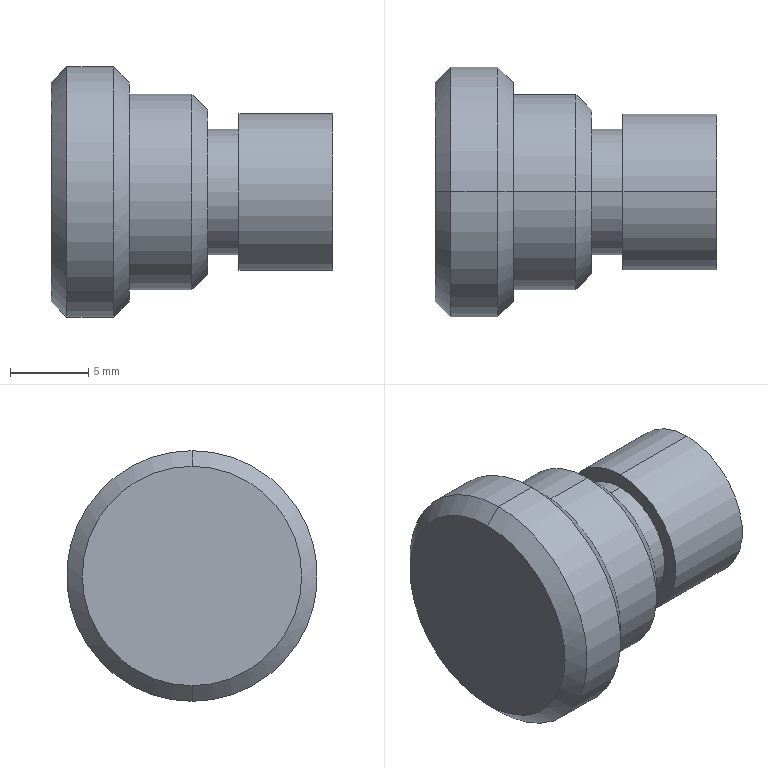Part | SolidWorks | features Chamfer 1, Revolution 1 | 1 solid | 19 faces | box 18 x 16 x 16 mm | volume 2124 mm3 | cylinder 8 | cone 6 | plane 5 | commonest cylinder face diameters 8 x2 10 x2 12.5 x2 16 x2
STEP:
#1=CARTESIAN_POINT('',(-124.445,-89.118,-5.25));
#2=VERTEX_POINT('',#1);
#3=CARTESIAN_POINT('',(-124.445,-89.118,5.25));
#4=VERTEX_POINT('',#3);
#5=CARTESIAN_POINT('',(-124.445,-89.118,0.));
#6=DIRECTION('',(1.,0.,0.));
#7=DIRECTION('',(0.,0.,1.));
#8=AXIS2_PLACEMENT_3D('',#5,#6,#7);
#9=CIRCLE('',#8,5.25);
#10=EDGE_CURVE('',#2,#4,#9,.T.);
#11=ORIENTED_EDGE('',*,*,#10,.F.);
#12=CARTESIAN_POINT('',(-125.445,-89.118,-6.25));
#13=VERTEX_POINT('',#12);
#14=CARTESIAN_POINT('',(-125.445,-89.118,-6.25));
#15=DIRECTION('',(-0.7071,0.,-0.7071));
#16=VECTOR('',#15,1000.);
#17=LINE('',#14,#16);
#18=EDGE_CURVE('',#2,#13,#17,.T.);
#19=ORIENTED_EDGE('',*,*,#18,.T.);
#20=CARTESIAN_POINT('',(-125.445,-89.118,6.25));
#21=VERTEX_POINT('',#20);
#22=CARTESIAN_POINT('',(-125.445,-89.118,0.));
#23=DIRECTION('',(-1.,0.,0.));
#24=DIRECTION('',(0.,0.,1.));
#25=AXIS2_PLACEMENT_3D('',#22,#23,#24);
#26=CIRCLE('',#25,6.25);
#27=EDGE_CURVE('',#21,#13,#26,.T.);
#28=ORIENTED_EDGE('',*,*,#27,.F.);
#29=CARTESIAN_POINT('',(-125.445,-89.118,6.25));
#30=DIRECTION('',(-0.7071,0.,0.7071));
#31=VECTOR('',#30,1000.);
#32=LINE('',#29,#31);
#33=EDGE_CURVE('',#4,#21,#32,.T.);
#34=ORIENTED_EDGE('',*,*,#33,.F.);
#35=EDGE_LOOP('',(#11,#19,#28,#34));
#36=FACE_OUTER_BOUND('',#35,.T.);
#37=CARTESIAN_POINT('',(-125.445,-89.118,0.));
#38=DIRECTION('',(-1.,0.,0.));
#39=DIRECTION('',(0.,0.,1.));
#40=AXIS2_PLACEMENT_3D('',#37,#38,#39);
#41=CONICAL_SURFACE('',#40,6.25,0.7854);
#42=ADVANCED_FACE('',(#36),#41,.T.);
#43=CARTESIAN_POINT('',(-129.445,-89.118,-7.));
#44=VERTEX_POINT('',#43);
#45=CARTESIAN_POINT('',(-129.445,-89.118,7.));
#46=VERTEX_POINT('',#45);
#47=CARTESIAN_POINT('',(-129.445,-89.118,0.));
#48=DIRECTION('',(1.,0.,0.));
#49=DIRECTION('',(0.,0.,1.));
#50=AXIS2_PLACEMENT_3D('',#47,#48,#49);
#51=CIRCLE('',#50,7.);
#52=EDGE_CURVE('',#44,#46,#51,.T.);
#53=ORIENTED_EDGE('',*,*,#52,.F.);
#54=CARTESIAN_POINT('',(-130.445,-89.118,-8.));
#55=VERTEX_POINT('',#54);
#56=CARTESIAN_POINT('',(-130.445,-89.118,-8.));
#57=DIRECTION('',(-0.7071,0.,-0.7071));
#58=VECTOR('',#57,1000.);
#59=LINE('',#56,#58);
#60=EDGE_CURVE('',#44,#55,#59,.T.);
#61=ORIENTED_EDGE('',*,*,#60,.T.);
#62=CARTESIAN_POINT('',(-130.445,-89.118,8.));
#63=VERTEX_POINT('',#62);
#64=CARTESIAN_POINT('',(-130.445,-89.118,0.));
#65=DIRECTION('',(-1.,0.,0.));
#66=DIRECTION('',(0.,0.,1.));
#67=AXIS2_PLACEMENT_3D('',#64,#65,#66);
#68=CIRCLE('',#67,8.);
#69=EDGE_CURVE('',#63,#55,#68,.T.);
#70=ORIENTED_EDGE('',*,*,#69,.F.);
#71=CARTESIAN_POINT('',(-130.445,-89.118,8.));
#72=DIRECTION('',(-0.7071,0.,0.7071));
#73=VECTOR('',#72,1000.);
#74=LINE('',#71,#73);
#75=EDGE_CURVE('',#46,#63,#74,.T.);
#76=ORIENTED_EDGE('',*,*,#75,.F.);
#77=EDGE_LOOP('',(#53,#61,#70,#76));
#78=FACE_OUTER_BOUND('',#77,.T.);
#79=CARTESIAN_POINT('',(-130.445,-89.118,0.));
#80=DIRECTION('',(-1.,0.,0.));
#81=DIRECTION('',(0.,0.,1.));
#82=AXIS2_PLACEMENT_3D('',#79,#80,#81);
#83=CONICAL_SURFACE('',#82,8.,0.7854);
#84=ADVANCED_FACE('',(#78),#83,.T.);
#85=CARTESIAN_POINT('',(-134.445,-89.118,7.));
#86=VERTEX_POINT('',#85);
#87=CARTESIAN_POINT('',(-134.445,-89.118,-7.));
#88=VERTEX_POINT('',#87);
#89=CARTESIAN_POINT('',(-134.445,-89.118,0.));
#90=DIRECTION('',(-1.,0.,0.));
#91=DIRECTION('',(0.,0.,-1.));
#92=AXIS2_PLACEMENT_3D('',#89,#90,#91);
#93=CIRCLE('',#92,7.);
#94=EDGE_CURVE('',#86,#88,#93,.T.);
#95=ORIENTED_EDGE('',*,*,#94,.F.);
#96=CARTESIAN_POINT('',(-133.445,-89.118,8.));
#97=VERTEX_POINT('',#96);
#98=CARTESIAN_POINT('',(-134.445,-89.118,7.));
#99=DIRECTION('',(0.7071,0.,0.7071));
#100=VECTOR('',#99,1000.);
#101=LINE('',#98,#100);
#102=EDGE_CURVE('',#86,#97,#101,.T.);
#103=ORIENTED_EDGE('',*,*,#102,.T.);
#104=CARTESIAN_POINT('',(-133.445,-89.118,-8.));
#105=VERTEX_POINT('',#104);
#106=CARTESIAN_POINT('',(-133.445,-89.118,0.));
#107=DIRECTION('',(1.,0.,0.));
#108=DIRECTION('',(0.,0.,-1.));
#109=AXIS2_PLACEMENT_3D('',#106,#107,#108);
#110=CIRCLE('',#109,8.);
#111=EDGE_CURVE('',#105,#97,#110,.T.);
#112=ORIENTED_EDGE('',*,*,#111,.F.);
#113=CARTESIAN_POINT('',(-134.445,-89.118,-7.));
#114=DIRECTION('',(0.7071,0.,-0.7071));
#115=VECTOR('',#114,1000.);
#116=LINE('',#113,#115);
#117=EDGE_CURVE('',#88,#105,#116,.T.);
#118=ORIENTED_EDGE('',*,*,#117,.F.);
#119=EDGE_LOOP('',(#95,#103,#112,#118));
#120=FACE_OUTER_BOUND('',#119,.T.);
#121=CARTESIAN_POINT('',(-134.445,-89.118,0.));
#122=DIRECTION('',(1.,0.,0.));
#123=DIRECTION('',(0.,0.,-1.));
#124=AXIS2_PLACEMENT_3D('',#121,#122,#123);
#125=CONICAL_SURFACE('',#124,7.,0.7854);
#126=ADVANCED_FACE('',(#120),#125,.T.);
#127=ORIENTED_EDGE('',*,*,#69,.T.);
#128=CARTESIAN_POINT('',(-129.445,-89.118,-8.));
#129=DIRECTION('',(-1.,0.,0.));
#130=VECTOR('',#129,1000.);
#131=LINE('',#128,#130);
#132=EDGE_CURVE('',#55,#105,#131,.T.);
#133=ORIENTED_EDGE('',*,*,#132,.T.);
#134=ORIENTED_EDGE('',*,*,#111,.T.);
#135=CARTESIAN_POINT('',(-129.445,-89.118,8.));
#136=DIRECTION('',(-1.,0.,0.));
#137=VECTOR('',#136,1000.);
#138=LINE('',#135,#137);
#139=EDGE_CURVE('',#63,#97,#138,.T.);
#140=ORIENTED_EDGE('',*,*,#139,.F.);
#141=EDGE_LOOP('',(#127,#133,#134,#140));
#142=FACE_OUTER_BOUND('',#141,.T.);
#143=CARTESIAN_POINT('',(-129.445,-89.118,0.));
#144=DIRECTION('',(-1.,0.,0.));
#145=DIRECTION('',(0.,0.,1.));
#146=AXIS2_PLACEMENT_3D('',#143,#144,#145);
#147=CYLINDRICAL_SURFACE('',#146,8.);
#148=ADVANCED_FACE('',(#142),#147,.T.);
#149=ORIENTED_EDGE('',*,*,#27,.T.);
#150=CARTESIAN_POINT('',(-129.445,-89.118,-6.25));
#151=VERTEX_POINT('',#150);
#152=CARTESIAN_POINT('',(-129.445,-89.118,-6.25));
#153=DIRECTION('',(-1.,0.,0.));
#154=VECTOR('',#153,1000.);
#155=LINE('',#152,#154);
#156=EDGE_CURVE('',#13,#151,#155,.T.);
#157=ORIENTED_EDGE('',*,*,#156,.T.);
#158=CARTESIAN_POINT('',(-129.445,-89.118,6.25));
#159=VERTEX_POINT('',#158);
#160=CARTESIAN_POINT('',(-129.445,-89.118,0.));
#161=DIRECTION('',(-1.,0.,0.));
#162=DIRECTION('',(0.,0.,1.));
#163=AXIS2_PLACEMENT_3D('',#160,#161,#162);
#164=CIRCLE('',#163,6.25);
#165=EDGE_CURVE('',#159,#151,#164,.T.);
#166=ORIENTED_EDGE('',*,*,#165,.F.);
#167=CARTESIAN_POINT('',(-129.445,-89.118,6.25));
#168=DIRECTION('',(-1.,0.,0.));
#169=VECTOR('',#168,1000.);
#170=LINE('',#167,#169);
#171=EDGE_CURVE('',#21,#159,#170,.T.);
#172=ORIENTED_EDGE('',*,*,#171,.F.);
#173=EDGE_LOOP('',(#149,#157,#166,#172));
#174=FACE_OUTER_BOUND('',#173,.T.);
#175=CARTESIAN_POINT('',(-129.445,-89.118,0.));
#176=DIRECTION('',(-1.,0.,0.));
#177=DIRECTION('',(0.,0.,1.));
#178=AXIS2_PLACEMENT_3D('',#175,#176,#177);
#179=CYLINDRICAL_SURFACE('',#178,6.25);
#180=ADVANCED_FACE('',(#174),#179,.T.);
#181=CARTESIAN_POINT('',(-122.445,-89.118,4.));
#182=VERTEX_POINT('',#181);
#183=CARTESIAN_POINT('',(-122.445,-89.118,-4.));
#184=VERTEX_POINT('',#183);
#185=CARTESIAN_POINT('',(-122.445,-89.118,0.));
#186=DIRECTION('',(-1.,0.,0.));
#187=DIRECTION('',(0.,0.,1.));
#188=AXIS2_PLACEMENT_3D('',#185,#186,#187);
#189=CIRCLE('',#188,4.);
#190=EDGE_CURVE('',#182,#184,#189,.T.);
#191=ORIENTED_EDGE('',*,*,#190,.T.);
#192=CARTESIAN_POINT('',(-124.445,-89.118,-4.));
#193=VERTEX_POINT('',#192);
#194=CARTESIAN_POINT('',(-129.445,-89.118,-4.));
#195=DIRECTION('',(-1.,0.,0.));
#196=VECTOR('',#195,1000.);
#197=LINE('',#194,#196);
#198=EDGE_CURVE('',#184,#193,#197,.T.);
#199=ORIENTED_EDGE('',*,*,#198,.T.);
#200=CARTESIAN_POINT('',(-124.445,-89.118,4.));
#201=VERTEX_POINT('',#200);
#202=CARTESIAN_POINT('',(-124.445,-89.118,0.));
#203=DIRECTION('',(-1.,0.,0.));
#204=DIRECTION('',(0.,0.,1.));
#205=AXIS2_PLACEMENT_3D('',#202,#203,#204);
#206=CIRCLE('',#205,4.);
#207=EDGE_CURVE('',#201,#193,#206,.T.);
#208=ORIENTED_EDGE('',*,*,#207,.F.);
#209=CARTESIAN_POINT('',(-129.445,-89.118,4.));
#210=DIRECTION('',(-1.,0.,0.));
#211=VECTOR('',#210,1000.);
#212=LINE('',#209,#211);
#213=EDGE_CURVE('',#182,#201,#212,.T.);
#214=ORIENTED_EDGE('',*,*,#213,.F.);
#215=EDGE_LOOP('',(#191,#199,#208,#214));
#216=FACE_OUTER_BOUND('',#215,.T.);
#217=CARTESIAN_POINT('',(-129.445,-89.118,0.));
#218=DIRECTION('',(-1.,0.,0.));
#219=DIRECTION('',(0.,0.,1.));
#220=AXIS2_PLACEMENT_3D('',#217,#218,#219);
#221=CYLINDRICAL_SURFACE('',#220,4.);
#222=ADVANCED_FACE('',(#216),#221,.T.);
#223=CARTESIAN_POINT('',(-116.445,-89.118,5.));
#224=VERTEX_POINT('',#223);
#225=CARTESIAN_POINT('',(-116.445,-89.118,-5.));
#226=VERTEX_POINT('',#225);
#227=CARTESIAN_POINT('',(-116.445,-89.118,0.));
#228=DIRECTION('',(-1.,0.,0.));
#229=DIRECTION('',(0.,0.,1.));
#230=AXIS2_PLACEMENT_3D('',#227,#228,#229);
#231=CIRCLE('',#230,5.);
#232=EDGE_CURVE('',#224,#226,#231,.T.);
#233=ORIENTED_EDGE('',*,*,#232,.T.);
#234=CARTESIAN_POINT('',(-122.445,-89.118,-5.));
#235=VERTEX_POINT('',#234);
#236=CARTESIAN_POINT('',(-129.445,-89.118,-5.));
#237=DIRECTION('',(-1.,0.,0.));
#238=VECTOR('',#237,1000.);
#239=LINE('',#236,#238);
#240=EDGE_CURVE('',#226,#235,#239,.T.);
#241=ORIENTED_EDGE('',*,*,#240,.T.);
#242=CARTESIAN_POINT('',(-122.445,-89.118,5.));
#243=VERTEX_POINT('',#242);
#244=CARTESIAN_POINT('',(-122.445,-89.118,0.));
#245=DIRECTION('',(-1.,0.,0.));
#246=DIRECTION('',(0.,0.,1.));
#247=AXIS2_PLACEMENT_3D('',#244,#245,#246);
#248=CIRCLE('',#247,5.);
#249=EDGE_CURVE('',#243,#235,#248,.T.);
#250=ORIENTED_EDGE('',*,*,#249,.F.);
#251=CARTESIAN_POINT('',(-129.445,-89.118,5.));
#252=DIRECTION('',(-1.,0.,0.));
#253=VECTOR('',#252,1000.);
#254=LINE('',#251,#253);
#255=EDGE_CURVE('',#224,#243,#254,.T.);
#256=ORIENTED_EDGE('',*,*,#255,.F.);
#257=EDGE_LOOP('',(#233,#241,#250,#256));
#258=FACE_OUTER_BOUND('',#257,.T.);
#259=CARTESIAN_POINT('',(-129.445,-89.118,0.));
#260=DIRECTION('',(-1.,0.,0.));
#261=DIRECTION('',(0.,0.,1.));
#262=AXIS2_PLACEMENT_3D('',#259,#260,#261);
#263=CYLINDRICAL_SURFACE('',#262,5.);
#264=ADVANCED_FACE('',(#258),#263,.T.);
#265=ORIENTED_EDGE('',*,*,#232,.F.);
#266=CARTESIAN_POINT('',(-116.445,-89.118,0.));
#267=DIRECTION('',(-1.,0.,0.));
#268=DIRECTION('',(0.,0.,1.));
#269=AXIS2_PLACEMENT_3D('',#266,#267,#268);
#270=CIRCLE('',#269,5.);
#271=EDGE_CURVE('',#226,#224,#270,.T.);
#272=ORIENTED_EDGE('',*,*,#271,.F.);
#273=EDGE_LOOP('',(#265,#272));
#274=FACE_OUTER_BOUND('',#273,.T.);
#275=CARTESIAN_POINT('',(-116.445,-84.118,0.));
#276=DIRECTION('',(-1.,0.,0.));
#277=DIRECTION('',(0.,0.,1.));
#278=AXIS2_PLACEMENT_3D('',#275,#276,#277);
#279=PLANE('',#278);
#280=ADVANCED_FACE('',(#274),#279,.F.);
#281=ORIENTED_EDGE('',*,*,#240,.F.);
#282=ORIENTED_EDGE('',*,*,#271,.T.);
#283=ORIENTED_EDGE('',*,*,#255,.T.);
#284=CARTESIAN_POINT('',(-122.445,-89.118,0.));
#285=DIRECTION('',(-1.,0.,0.));
#286=DIRECTION('',(0.,0.,1.));
#287=AXIS2_PLACEMENT_3D('',#284,#285,#286);
#288=CIRCLE('',#287,5.);
#289=EDGE_CURVE('',#235,#243,#288,.T.);
#290=ORIENTED_EDGE('',*,*,#289,.F.);
#291=EDGE_LOOP('',(#281,#282,#283,#290));
#292=FACE_OUTER_BOUND('',#291,.T.);
#293=CARTESIAN_POINT('',(-129.445,-89.118,0.));
#294=DIRECTION('',(-1.,0.,0.));
#295=DIRECTION('',(0.,0.,1.));
#296=AXIS2_PLACEMENT_3D('',#293,#294,#295);
#297=CYLINDRICAL_SURFACE('',#296,5.);
#298=ADVANCED_FACE('',(#292),#297,.T.);
#299=ORIENTED_EDGE('',*,*,#190,.F.);
#300=CARTESIAN_POINT('',(-122.445,-89.118,0.));
#301=DIRECTION('',(-1.,0.,0.));
#302=DIRECTION('',(0.,0.,1.));
#303=AXIS2_PLACEMENT_3D('',#300,#301,#302);
#304=CIRCLE('',#303,4.);
#305=EDGE_CURVE('',#184,#182,#304,.T.);
#306=ORIENTED_EDGE('',*,*,#305,.F.);
#307=EDGE_LOOP('',(#299,#306));
#308=FACE_BOUND('',#307,.T.);
#309=ORIENTED_EDGE('',*,*,#249,.T.);
#310=ORIENTED_EDGE('',*,*,#289,.T.);
#311=EDGE_LOOP('',(#309,#310));
#312=FACE_OUTER_BOUND('',#311,.T.);
#313=CARTESIAN_POINT('',(-122.445,-84.118,0.));
#314=DIRECTION('',(1.,0.,0.));
#315=DIRECTION('',(0.,0.,-1.));
#316=AXIS2_PLACEMENT_3D('',#313,#314,#315);
#317=PLANE('',#316);
#318=ADVANCED_FACE('',(#308,#312),#317,.F.);
#319=ORIENTED_EDGE('',*,*,#198,.F.);
#320=ORIENTED_EDGE('',*,*,#305,.T.);
#321=ORIENTED_EDGE('',*,*,#213,.T.);
#322=CARTESIAN_POINT('',(-124.445,-89.118,0.));
#323=DIRECTION('',(-1.,0.,0.));
#324=DIRECTION('',(0.,0.,1.));
#325=AXIS2_PLACEMENT_3D('',#322,#323,#324);
#326=CIRCLE('',#325,4.);
#327=EDGE_CURVE('',#193,#201,#326,.T.);
#328=ORIENTED_EDGE('',*,*,#327,.F.);
#329=EDGE_LOOP('',(#319,#320,#321,#328));
#330=FACE_OUTER_BOUND('',#329,.T.);
#331=CARTESIAN_POINT('',(-129.445,-89.118,0.));
#332=DIRECTION('',(-1.,0.,0.));
#333=DIRECTION('',(0.,0.,1.));
#334=AXIS2_PLACEMENT_3D('',#331,#332,#333);
#335=CYLINDRICAL_SURFACE('',#334,4.);
#336=ADVANCED_FACE('',(#330),#335,.T.);
#337=CARTESIAN_POINT('',(-124.445,-89.118,0.));
#338=DIRECTION('',(1.,0.,0.));
#339=DIRECTION('',(0.,0.,1.));
#340=AXIS2_PLACEMENT_3D('',#337,#338,#339);
#341=CIRCLE('',#340,5.25);
#342=EDGE_CURVE('',#4,#2,#341,.T.);
#343=ORIENTED_EDGE('',*,*,#342,.T.);
#344=ORIENTED_EDGE('',*,*,#10,.T.);
#345=EDGE_LOOP('',(#343,#344));
#346=FACE_OUTER_BOUND('',#345,.T.);
#347=ORIENTED_EDGE('',*,*,#207,.T.);
#348=ORIENTED_EDGE('',*,*,#327,.T.);
#349=EDGE_LOOP('',(#347,#348));
#350=FACE_BOUND('',#349,.T.);
#351=CARTESIAN_POINT('',(-124.445,-85.118,0.));
#352=DIRECTION('',(-1.,0.,0.));
#353=DIRECTION('',(0.,0.,1.));
#354=AXIS2_PLACEMENT_3D('',#351,#352,#353);
#355=PLANE('',#354);
#356=ADVANCED_FACE('',(#346,#350),#355,.F.);
#357=ORIENTED_EDGE('',*,*,#156,.F.);
#358=CARTESIAN_POINT('',(-125.445,-89.118,0.));
#359=DIRECTION('',(-1.,0.,0.));
#360=DIRECTION('',(0.,0.,1.));
#361=AXIS2_PLACEMENT_3D('',#358,#359,#360);
#362=CIRCLE('',#361,6.25);
#363=EDGE_CURVE('',#13,#21,#362,.T.);
#364=ORIENTED_EDGE('',*,*,#363,.T.);
#365=ORIENTED_EDGE('',*,*,#171,.T.);
#366=CARTESIAN_POINT('',(-129.445,-89.118,0.));
#367=DIRECTION('',(-1.,0.,0.));
#368=DIRECTION('',(0.,0.,1.));
#369=AXIS2_PLACEMENT_3D('',#366,#367,#368);
#370=CIRCLE('',#369,6.25);
#371=EDGE_CURVE('',#151,#159,#370,.T.);
#372=ORIENTED_EDGE('',*,*,#371,.F.);
#373=EDGE_LOOP('',(#357,#364,#365,#372));
#374=FACE_OUTER_BOUND('',#373,.T.);
#375=CARTESIAN_POINT('',(-129.445,-89.118,0.));
#376=DIRECTION('',(-1.,0.,0.));
#377=DIRECTION('',(0.,0.,1.));
#378=AXIS2_PLACEMENT_3D('',#375,#376,#377);
#379=CYLINDRICAL_SURFACE('',#378,6.25);
#380=ADVANCED_FACE('',(#374),#379,.T.);
#381=CARTESIAN_POINT('',(-129.445,-89.118,0.));
#382=DIRECTION('',(1.,0.,0.));
#383=DIRECTION('',(0.,0.,1.));
#384=AXIS2_PLACEMENT_3D('',#381,#382,#383);
#385=CIRCLE('',#384,7.);
#386=EDGE_CURVE('',#46,#44,#385,.T.);
#387=ORIENTED_EDGE('',*,*,#386,.T.);
#388=ORIENTED_EDGE('',*,*,#52,.T.);
#389=EDGE_LOOP('',(#387,#388));
#390=FACE_OUTER_BOUND('',#389,.T.);
#391=ORIENTED_EDGE('',*,*,#165,.T.);
#392=ORIENTED_EDGE('',*,*,#371,.T.);
#393=EDGE_LOOP('',(#391,#392));
#394=FACE_BOUND('',#393,.T.);
#395=CARTESIAN_POINT('',(-129.445,-82.868,0.));
#396=DIRECTION('',(-1.,0.,0.));
#397=DIRECTION('',(0.,0.,1.));
#398=AXIS2_PLACEMENT_3D('',#395,#396,#397);
#399=PLANE('',#398);
#400=ADVANCED_FACE('',(#390,#394),#399,.F.);
#401=ORIENTED_EDGE('',*,*,#132,.F.);
#402=CARTESIAN_POINT('',(-130.445,-89.118,0.));
#403=DIRECTION('',(-1.,0.,0.));
#404=DIRECTION('',(0.,0.,1.));
#405=AXIS2_PLACEMENT_3D('',#402,#403,#404);
#406=CIRCLE('',#405,8.);
#407=EDGE_CURVE('',#55,#63,#406,.T.);
#408=ORIENTED_EDGE('',*,*,#407,.T.);
#409=ORIENTED_EDGE('',*,*,#139,.T.);
#410=CARTESIAN_POINT('',(-133.445,-89.118,0.));
#411=DIRECTION('',(1.,0.,0.));
#412=DIRECTION('',(0.,0.,-1.));
#413=AXIS2_PLACEMENT_3D('',#410,#411,#412);
#414=CIRCLE('',#413,8.);
#415=EDGE_CURVE('',#97,#105,#414,.T.);
#416=ORIENTED_EDGE('',*,*,#415,.T.);
#417=EDGE_LOOP('',(#401,#408,#409,#416));
#418=FACE_OUTER_BOUND('',#417,.T.);
#419=CARTESIAN_POINT('',(-129.445,-89.118,0.));
#420=DIRECTION('',(-1.,0.,0.));
#421=DIRECTION('',(0.,0.,1.));
#422=AXIS2_PLACEMENT_3D('',#419,#420,#421);
#423=CYLINDRICAL_SURFACE('',#422,8.);
#424=ADVANCED_FACE('',(#418),#423,.T.);
#425=CARTESIAN_POINT('',(-134.445,-89.118,0.));
#426=DIRECTION('',(-1.,0.,0.));
#427=DIRECTION('',(0.,0.,-1.));
#428=AXIS2_PLACEMENT_3D('',#425,#426,#427);
#429=CIRCLE('',#428,7.);
#430=EDGE_CURVE('',#88,#86,#429,.T.);
#431=ORIENTED_EDGE('',*,*,#430,.T.);
#432=ORIENTED_EDGE('',*,*,#94,.T.);
#433=EDGE_LOOP('',(#431,#432));
#434=FACE_OUTER_BOUND('',#433,.T.);
#435=CARTESIAN_POINT('',(-134.445,-81.118,0.));
#436=DIRECTION('',(1.,0.,0.));
#437=DIRECTION('',(0.,0.,-1.));
#438=AXIS2_PLACEMENT_3D('',#435,#436,#437);
#439=PLANE('',#438);
#440=ADVANCED_FACE('',(#434),#439,.F.);
#441=ORIENTED_EDGE('',*,*,#102,.F.);
#442=ORIENTED_EDGE('',*,*,#430,.F.);
#443=ORIENTED_EDGE('',*,*,#117,.T.);
#444=ORIENTED_EDGE('',*,*,#415,.F.);
#445=EDGE_LOOP('',(#441,#442,#443,#444));
#446=FACE_OUTER_BOUND('',#445,.T.);
#447=CARTESIAN_POINT('',(-134.445,-89.118,0.));
#448=DIRECTION('',(1.,0.,0.));
#449=DIRECTION('',(0.,0.,-1.));
#450=AXIS2_PLACEMENT_3D('',#447,#448,#449);
#451=CONICAL_SURFACE('',#450,7.,0.7854);
#452=ADVANCED_FACE('',(#446),#451,.T.);
#453=ORIENTED_EDGE('',*,*,#60,.F.);
#454=ORIENTED_EDGE('',*,*,#386,.F.);
#455=ORIENTED_EDGE('',*,*,#75,.T.);
#456=ORIENTED_EDGE('',*,*,#407,.F.);
#457=EDGE_LOOP('',(#453,#454,#455,#456));
#458=FACE_OUTER_BOUND('',#457,.T.);
#459=CARTESIAN_POINT('',(-130.445,-89.118,0.));
#460=DIRECTION('',(-1.,0.,0.));
#461=DIRECTION('',(0.,0.,1.));
#462=AXIS2_PLACEMENT_3D('',#459,#460,#461);
#463=CONICAL_SURFACE('',#462,8.,0.7854);
#464=ADVANCED_FACE('',(#458),#463,.T.);
#465=ORIENTED_EDGE('',*,*,#18,.F.);
#466=ORIENTED_EDGE('',*,*,#342,.F.);
#467=ORIENTED_EDGE('',*,*,#33,.T.);
#468=ORIENTED_EDGE('',*,*,#363,.F.);
#469=EDGE_LOOP('',(#465,#466,#467,#468));
#470=FACE_OUTER_BOUND('',#469,.T.);
#471=CARTESIAN_POINT('',(-125.445,-89.118,0.));
#472=DIRECTION('',(-1.,0.,0.));
#473=DIRECTION('',(0.,0.,1.));
#474=AXIS2_PLACEMENT_3D('',#471,#472,#473);
#475=CONICAL_SURFACE('',#474,6.25,0.7854);
#476=ADVANCED_FACE('',(#470),#475,.T.);
#477=CLOSED_SHELL('',(#42,#84,#126,#148,#180,#222,#264,#280,#298,#318,#336,#356,#380,#400,#424,#440,#452,#464,#476));
#478=MANIFOLD_SOLID_BREP('',#477);
#479=CARTESIAN_POINT('',(0.,0.,0.));
#480=DIRECTION('',(0.,0.,1.));
#481=DIRECTION('',(1.,0.,0.));
#482=AXIS2_PLACEMENT_3D('',#479,#480,#481);
#483=(LENGTH_UNIT()NAMED_UNIT(*)SI_UNIT(.MILLI.,.METRE.));
#484=UNCERTAINTY_MEASURE_WITH_UNIT(LENGTH_MEASURE(0.00001),#483,'','');
#485=(NAMED_UNIT(*)PLANE_ANGLE_UNIT()SI_UNIT($,.RADIAN.));
#486=(NAMED_UNIT(*)SI_UNIT($,.STERADIAN.)SOLID_ANGLE_UNIT());
#487=(GEOMETRIC_REPRESENTATION_CONTEXT(3)GLOBAL_UNCERTAINTY_ASSIGNED_CONTEXT((#484))GLOBAL_UNIT_ASSIGNED_CONTEXT((#483,#485,#486))REPRESENTATION_CONTEXT('',''));
#488=ADVANCED_BREP_SHAPE_REPRESENTATION('',(#478,#482),#487);